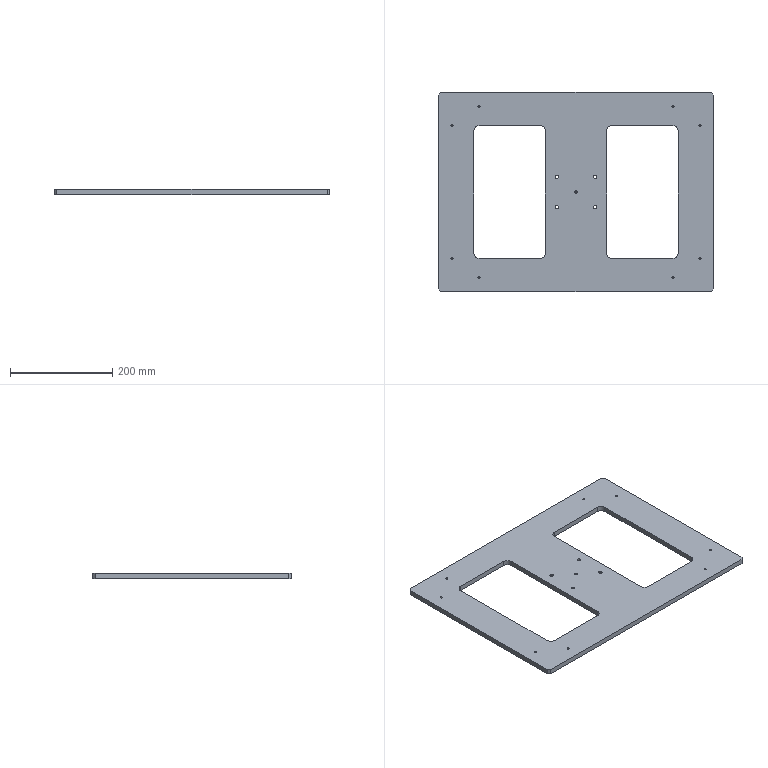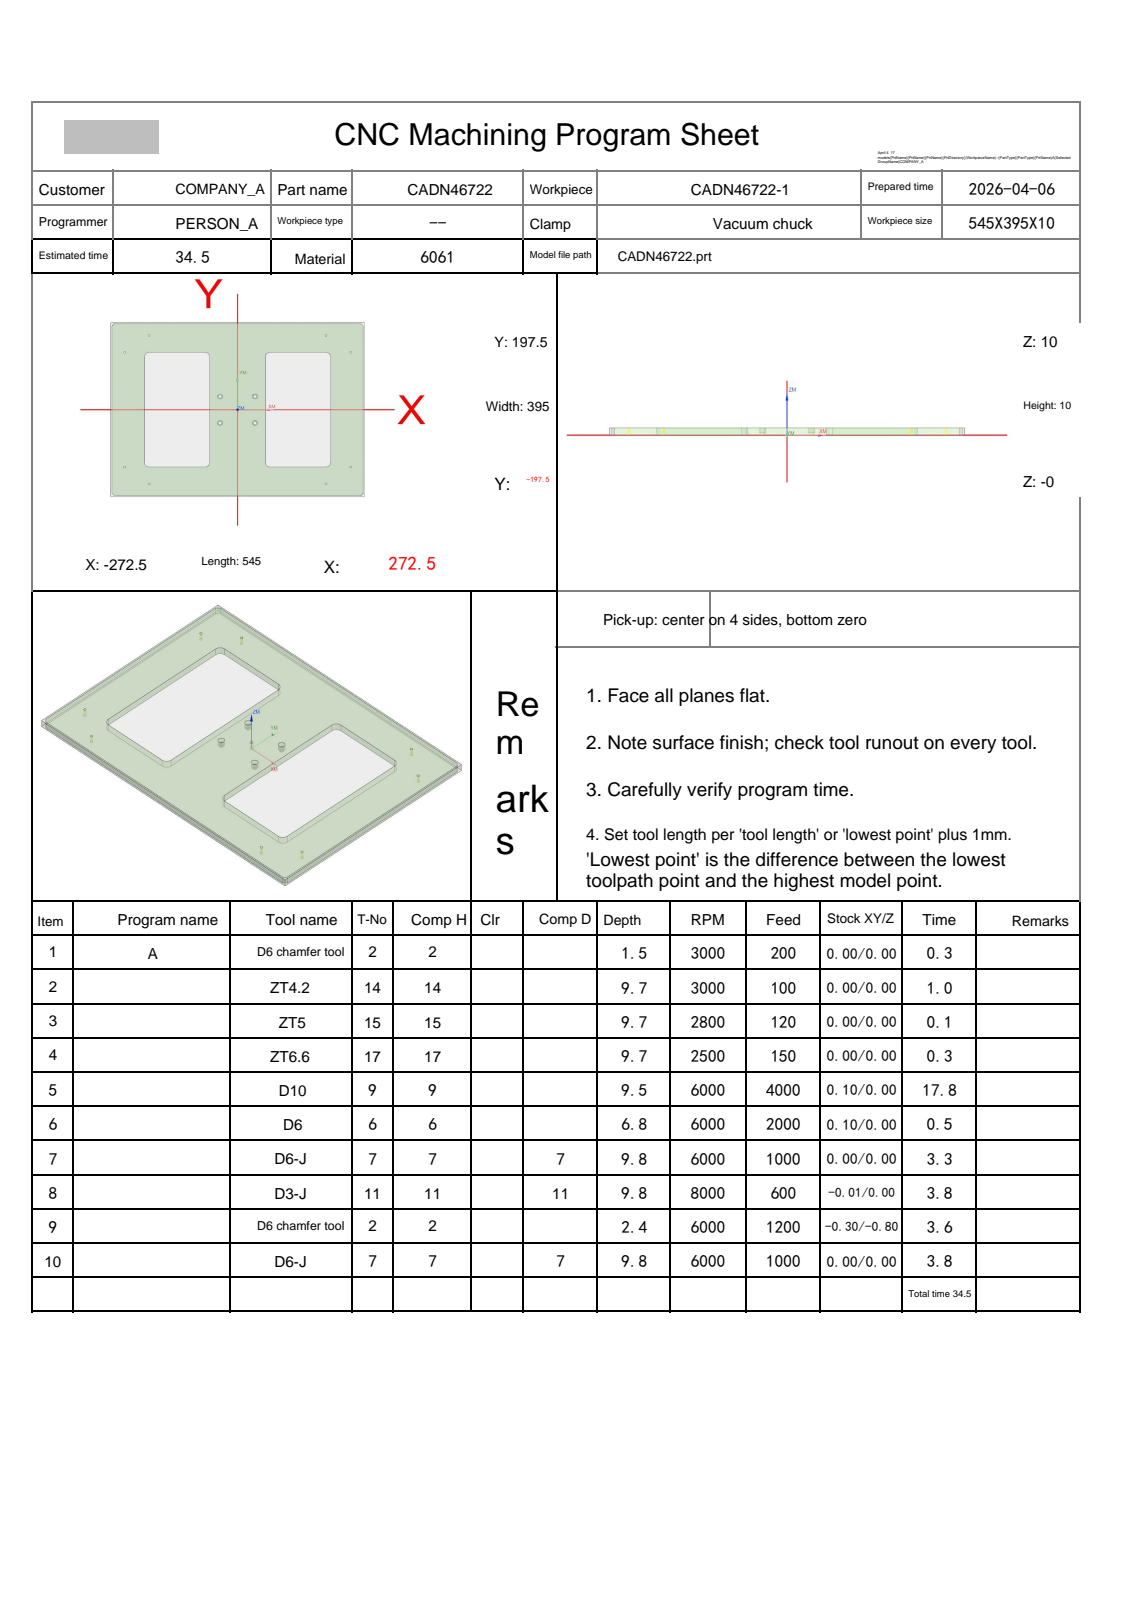NC program | NX | posted by the shop | part box 540 x 390 x 10 mm
Lines 1 to 1058 of 3473:
%
O0001
(Machine time: 36.48 MIN)
(===Total Tool:8===)
(T2=D6 chamfer tool   D=6.   R=0.   D-  H02 Z=7.63  )
(T14=ZT4.2  D=4.2  DR_a=118 D-  H14 Z=0.3   )
(T15=ZT5    D=5.   DR_a=118 D-  H15 Z=0.3   )
(T17=ZT6.6  D=6.6  DR_a=118 D-  H17 Z=0.3   )
(T9=D10     D=10.  R=0.   D-  H09 Z=0.5   )
(T6=D6      D=6.   R=0.   D-  H06 Z=3.2   )
(T7=D6-J    D=6.   R=0.   D7  H07 Z=0.2   )
(T11=D3-J   D=3.   R=0.   D11 H11 Z=0.2   )
G80 G90 G17 G49 G40
G91 G28 Z0
M01
N1 T02 M06
(D6 chamfer tool  D=6. R=0. H=02 ce=0.00 di=0.00)
G00 G90 G54 X190. Y-168. M03 S3000
G43 H02 Z30.
M08
G98 G81 X190. Y-168. Z8.5 R11. F200.
X243. Y-130.
Y130.
X190. Y168.
X37.5 Y30.
Y-30.
X0.0 Y0.0
X-37.5 Y30.
Y-30.
X-190. Y-168.
X-243. Y-130.
Y130.
X-190. Y168.
G80
G00 Z30.
G91 G28 Z0.0
M05
M09
G91 G28 Z0.0
M01
N2 T14 M06
(ZT4.2 D=4.2 DR_a=118 H=14)
G00 G90 G54 X190. Y-168. M03 S3000
G43 H14 Z30.
M08
G98 G83 X190. Y-168. Z.3 R11. F100. Q1.5
X243. Y-130.
Y130.
X190. Y168.
X-190.
X-243. Y130.
Y-130.
X-190. Y-168.
G80
G00 Z30.
G91 G28 Z0.0
M05
M09
G91 G28 Z0.0
M01
N3 T15 M06
(ZT5 D=5. DR_a=118 H=15)
G00 G90 G54 X0.0 Y0.0 M03 S2800
G43 H15 Z30.
M08
G98 G83 X0.0 Y0.0 Z.3 R11. F120. Q1.5
G80
G00 Z30.
G91 G28 Z0.0
M05
M09
G91 G28 Z0.0
M01
N4 T17 M06
(ZT6.6 D=6.6 DR_a=118 H=17)
G00 G90 G54 X-37.5 Y-30. M03 S2500
G43 H17 Z30.
M08
G98 G83 X-37.5 Y-30. Z.3 R11. F150. Q3.
Y30.
X37.5
Y-30.
G80
G00 Z30.
G91 G28 Z0.0
M05
M09
G91 G28 Z0.0
M01
N5 T09 M06
(D10  D=10. R=0. H=09 ce=0.10 di=0.00)
G00 G90 G54 X-194.9 Y0.0 M03 S6000
G43 H09 Z30.
M08
Z10.5
G01 Y-120. Z10.42 F4000.
G03 X-190. Y-124.9 Z10.415 I4.9 J0.0
G01 X-70. Z10.335
G03 X-65.1 Y-120. Z10.33 I0.0 J4.9
G01 Y120. Z10.17
G03 X-70. Y124.9 Z10.165 I-4.9 J0.0
G01 X-190. Z10.085
G03 X-194.9 Y120. Z10.08 I0.0 J-4.9
G01 Y-120. Z9.92
G03 X-190. Y-124.9 Z9.915 I4.9 J0.0
G01 X-70. Z9.835
G03 X-65.1 Y-120. Z9.83 I0.0 J4.9
G01 Y120. Z9.67
G03 X-70. Y124.9 Z9.665 I-4.9 J0.0
G01 X-190. Z9.585
G03 X-194.9 Y120. Z9.58 I0.0 J-4.9
G01 Y-120. Z9.42
G03 X-190. Y-124.9 Z9.415 I4.9 J0.0
G01 X-70. Z9.335
G03 X-65.1 Y-120. Z9.33 I0.0 J4.9
G01 Y120. Z9.17
G03 X-70. Y124.9 Z9.165 I-4.9 J0.0
G01 X-190. Z9.085
G03 X-194.9 Y120. Z9.08 I0.0 J-4.9
G01 Y-120. Z8.92
G03 X-190. Y-124.9 Z8.915 I4.9 J0.0
G01 X-70. Z8.835
G03 X-65.1 Y-120. Z8.83 I0.0 J4.9
G01 Y120. Z8.67
G03 X-70. Y124.9 Z8.665 I-4.9 J0.0
G01 X-190. Z8.585
G03 X-194.9 Y120. Z8.58 I0.0 J-4.9
G01 Y-120. Z8.42
G03 X-190. Y-124.9 Z8.415 I4.9 J0.0
G01 X-70. Z8.335
G03 X-65.1 Y-120. Z8.33 I0.0 J4.9
G01 Y120. Z8.17
G03 X-70. Y124.9 Z8.165 I-4.9 J0.0
G01 X-190. Z8.085
G03 X-194.9 Y120. Z8.08 I0.0 J-4.9
G01 Y-120. Z7.92
G03 X-190. Y-124.9 Z7.915 I4.9 J0.0
G01 X-70. Z7.835
G03 X-65.1 Y-120. Z7.83 I0.0 J4.9
G01 Y120. Z7.67
G03 X-70. Y124.9 Z7.665 I-4.9 J0.0
G01 X-190. Z7.585
G03 X-194.9 Y120. Z7.58 I0.0 J-4.9
G01 Y-120. Z7.42
G03 X-190. Y-124.9 Z7.415 I4.9 J0.0
G01 X-70. Z7.335
G03 X-65.1 Y-120. Z7.33 I0.0 J4.9
G01 Y120. Z7.17
G03 X-70. Y124.9 Z7.165 I-4.9 J0.0
G01 X-190. Z7.085
G03 X-194.9 Y120. Z7.08 I0.0 J-4.9
G01 Y-120. Z6.92
G03 X-190. Y-124.9 Z6.915 I4.9 J0.0
G01 X-70. Z6.835
G03 X-65.1 Y-120. Z6.83 I0.0 J4.9
G01 Y120. Z6.67
G03 X-70. Y124.9 Z6.665 I-4.9 J0.0
G01 X-190. Z6.585
G03 X-194.9 Y120. Z6.58 I0.0 J-4.9
G01 Y-120. Z6.42
G03 X-190. Y-124.9 Z6.415 I4.9 J0.0
G01 X-70. Z6.335
G03 X-65.1 Y-120. Z6.33 I0.0 J4.9
G01 Y120. Z6.17
G03 X-70. Y124.9 Z6.165 I-4.9 J0.0
G01 X-190. Z6.085
G03 X-194.9 Y120. Z6.08 I0.0 J-4.9
G01 Y-120. Z5.92
G03 X-190. Y-124.9 Z5.915 I4.9 J0.0
G01 X-70. Z5.835
G03 X-65.1 Y-120. Z5.83 I0.0 J4.9
G01 Y120. Z5.67
G03 X-70. Y124.9 Z5.665 I-4.9 J0.0
G01 X-190. Z5.585
G03 X-194.9 Y120. Z5.58 I0.0 J-4.9
G01 Y-120. Z5.42
G03 X-190. Y-124.9 Z5.415 I4.9 J0.0
G01 X-70. Z5.335
G03 X-65.1 Y-120. Z5.33 I0.0 J4.9
G01 Y120. Z5.17
G03 X-70. Y124.9 Z5.165 I-4.9 J0.0
G01 X-190. Z5.085
G03 X-194.9 Y120. Z5.08 I0.0 J-4.9
G01 Y-120. Z4.92
G03 X-190. Y-124.9 Z4.915 I4.9 J0.0
G01 X-70. Z4.835
G03 X-65.1 Y-120. Z4.83 I0.0 J4.9
G01 Y120. Z4.67
G03 X-70. Y124.9 Z4.665 I-4.9 J0.0
G01 X-190. Z4.585
G03 X-194.9 Y120. Z4.58 I0.0 J-4.9
G01 Y-120. Z4.42
G03 X-190. Y-124.9 Z4.415 I4.9 J0.0
G01 X-70. Z4.335
G03 X-65.1 Y-120. Z4.33 I0.0 J4.9
G01 Y120. Z4.17
G03 X-70. Y124.9 Z4.165 I-4.9 J0.0
G01 X-190. Z4.085
G03 X-194.9 Y120. Z4.08 I0.0 J-4.9
G01 Y-120. Z3.92
G03 X-190. Y-124.9 Z3.915 I4.9 J0.0
G01 X-70. Z3.835
G03 X-65.1 Y-120. Z3.83 I0.0 J4.9
G01 Y120. Z3.67
G03 X-70. Y124.9 Z3.665 I-4.9 J0.0
G01 X-190. Z3.585
G03 X-194.9 Y120. Z3.58 I0.0 J-4.9
G01 Y-120. Z3.42
G03 X-190. Y-124.9 Z3.415 I4.9 J0.0
G01 X-70. Z3.335
G03 X-65.1 Y-120. Z3.33 I0.0 J4.9
G01 Y120. Z3.17
G03 X-70. Y124.9 Z3.165 I-4.9 J0.0
G01 X-190. Z3.085
G03 X-194.9 Y120. Z3.08 I0.0 J-4.9
G01 Y-120. Z2.92
G03 X-190. Y-124.9 Z2.915 I4.9 J0.0
G01 X-70. Z2.835
G03 X-65.1 Y-120. Z2.83 I0.0 J4.9
G01 Y120. Z2.67
G03 X-70. Y124.9 Z2.665 I-4.9 J0.0
G01 X-190. Z2.585
G03 X-194.9 Y120. Z2.58 I0.0 J-4.9
G01 Y-120. Z2.42
G03 X-190. Y-124.9 Z2.415 I4.9 J0.0
G01 X-70. Z2.335
G03 X-65.1 Y-120. Z2.33 I0.0 J4.9
G01 Y120. Z2.17
G03 X-70. Y124.9 Z2.165 I-4.9 J0.0
G01 X-190. Z2.085
G03 X-194.9 Y120. Z2.08 I0.0 J-4.9
G01 Y-120. Z1.92
G03 X-190. Y-124.9 Z1.915 I4.9 J0.0
G01 X-70. Z1.835
G03 X-65.1 Y-120. Z1.83 I0.0 J4.9
G01 Y120. Z1.67
G03 X-70. Y124.9 Z1.665 I-4.9 J0.0
G01 X-190. Z1.585
G03 X-194.9 Y120. Z1.58 I0.0 J-4.9
G01 Y-120. Z1.42
G03 X-190. Y-124.9 Z1.415 I4.9 J0.0
G01 X-70. Z1.335
G03 X-65.1 Y-120. Z1.33 I0.0 J4.9
G01 Y120. Z1.17
G03 X-70. Y124.9 Z1.165 I-4.9 J0.0
G01 X-190. Z1.085
G03 X-194.9 Y120. Z1.08 I0.0 J-4.9
G01 Y-120. Z.92
G03 X-190. Y-124.9 Z.915 I4.9 J0.0
G01 X-70. Z.835
G03 X-65.1 Y-120. Z.83 I0.0 J4.9
G01 Y120. Z.67
G03 X-70. Y124.9 Z.665 I-4.9 J0.0
G01 X-190. Z.585
G03 X-194.9 Y120. Z.58 I0.0 J-4.9
G01 Y0.0 Z.5
Y-120.
G03 X-190. Y-124.9 I4.9 J0.0
G01 X-70.
G03 X-65.1 Y-120. I0.0 J4.9
G01 Y120.
G03 X-70. Y124.9 I-4.9 J0.0
G01 X-190.
G03 X-194.9 Y120. I0.0 J-4.9
G01 Y0.0
Y-.5
Z1.5
G00 Z30.
X194.9 Y0.0
Z10.5
G01 Y120. Z10.42
G03 X190. Y124.9 Z10.415 I-4.9 J0.0
G01 X70. Z10.335
G03 X65.1 Y120. Z10.33 I0.0 J-4.9
G01 Y-120. Z10.17
G03 X70. Y-124.9 Z10.165 I4.9 J0.0
G01 X190. Z10.085
G03 X194.9 Y-120. Z10.08 I0.0 J4.9
G01 Y120. Z9.92
G03 X190. Y124.9 Z9.915 I-4.9 J0.0
G01 X70. Z9.835
G03 X65.1 Y120. Z9.83 I0.0 J-4.9
G01 Y-120. Z9.67
G03 X70. Y-124.9 Z9.665 I4.9 J0.0
G01 X190. Z9.585
G03 X194.9 Y-120. Z9.58 I0.0 J4.9
G01 Y120. Z9.42
G03 X190. Y124.9 Z9.415 I-4.9 J0.0
G01 X70. Z9.335
G03 X65.1 Y120. Z9.33 I0.0 J-4.9
G01 Y-120. Z9.17
G03 X70. Y-124.9 Z9.165 I4.9 J0.0
G01 X190. Z9.085
G03 X194.9 Y-120. Z9.08 I0.0 J4.9
G01 Y120. Z8.92
G03 X190. Y124.9 Z8.915 I-4.9 J0.0
G01 X70. Z8.835
G03 X65.1 Y120. Z8.83 I0.0 J-4.9
G01 Y-120. Z8.67
G03 X70. Y-124.9 Z8.665 I4.9 J0.0
G01 X190. Z8.585
G03 X194.9 Y-120. Z8.58 I0.0 J4.9
G01 Y120. Z8.42
G03 X190. Y124.9 Z8.415 I-4.9 J0.0
G01 X70. Z8.335
G03 X65.1 Y120. Z8.33 I0.0 J-4.9
G01 Y-120. Z8.17
G03 X70. Y-124.9 Z8.165 I4.9 J0.0
G01 X190. Z8.085
G03 X194.9 Y-120. Z8.08 I0.0 J4.9
G01 Y120. Z7.92
G03 X190. Y124.9 Z7.915 I-4.9 J0.0
G01 X70. Z7.835
G03 X65.1 Y120. Z7.83 I0.0 J-4.9
G01 Y-120. Z7.67
G03 X70. Y-124.9 Z7.665 I4.9 J0.0
G01 X190. Z7.585
G03 X194.9 Y-120. Z7.58 I0.0 J4.9
G01 Y120. Z7.42
G03 X190. Y124.9 Z7.415 I-4.9 J0.0
G01 X70. Z7.335
G03 X65.1 Y120. Z7.33 I0.0 J-4.9
G01 Y-120. Z7.17
G03 X70. Y-124.9 Z7.165 I4.9 J0.0
G01 X190. Z7.085
G03 X194.9 Y-120. Z7.08 I0.0 J4.9
G01 Y120. Z6.92
G03 X190. Y124.9 Z6.915 I-4.9 J0.0
G01 X70. Z6.835
G03 X65.1 Y120. Z6.83 I0.0 J-4.9
G01 Y-120. Z6.67
G03 X70. Y-124.9 Z6.665 I4.9 J0.0
G01 X190. Z6.585
G03 X194.9 Y-120. Z6.58 I0.0 J4.9
G01 Y120. Z6.42
G03 X190. Y124.9 Z6.415 I-4.9 J0.0
G01 X70. Z6.335
G03 X65.1 Y120. Z6.33 I0.0 J-4.9
G01 Y-120. Z6.17
G03 X70. Y-124.9 Z6.165 I4.9 J0.0
G01 X190. Z6.085
G03 X194.9 Y-120. Z6.08 I0.0 J4.9
G01 Y120. Z5.92
G03 X190. Y124.9 Z5.915 I-4.9 J0.0
G01 X70. Z5.835
G03 X65.1 Y120. Z5.83 I0.0 J-4.9
G01 Y-120. Z5.67
G03 X70. Y-124.9 Z5.665 I4.9 J0.0
G01 X190. Z5.585
G03 X194.9 Y-120. Z5.58 I0.0 J4.9
G01 Y120. Z5.42
G03 X190. Y124.9 Z5.415 I-4.9 J0.0
G01 X70. Z5.335
G03 X65.1 Y120. Z5.33 I0.0 J-4.9
G01 Y-120. Z5.17
G03 X70. Y-124.9 Z5.165 I4.9 J0.0
G01 X190. Z5.085
G03 X194.9 Y-120. Z5.08 I0.0 J4.9
G01 Y120. Z4.92
G03 X190. Y124.9 Z4.915 I-4.9 J0.0
G01 X70. Z4.835
G03 X65.1 Y120. Z4.83 I0.0 J-4.9
G01 Y-120. Z4.67
G03 X70. Y-124.9 Z4.665 I4.9 J0.0
G01 X190. Z4.585
G03 X194.9 Y-120. Z4.58 I0.0 J4.9
G01 Y120. Z4.42
G03 X190. Y124.9 Z4.415 I-4.9 J0.0
G01 X70. Z4.335
G03 X65.1 Y120. Z4.33 I0.0 J-4.9
G01 Y-120. Z4.17
G03 X70. Y-124.9 Z4.165 I4.9 J0.0
G01 X190. Z4.085
G03 X194.9 Y-120. Z4.08 I0.0 J4.9
G01 Y120. Z3.92
G03 X190. Y124.9 Z3.915 I-4.9 J0.0
G01 X70. Z3.835
G03 X65.1 Y120. Z3.83 I0.0 J-4.9
G01 Y-120. Z3.67
G03 X70. Y-124.9 Z3.665 I4.9 J0.0
G01 X190. Z3.585
G03 X194.9 Y-120. Z3.58 I0.0 J4.9
G01 Y120. Z3.42
G03 X190. Y124.9 Z3.415 I-4.9 J0.0
G01 X70. Z3.335
G03 X65.1 Y120. Z3.33 I0.0 J-4.9
G01 Y-120. Z3.17
G03 X70. Y-124.9 Z3.165 I4.9 J0.0
G01 X190. Z3.085
G03 X194.9 Y-120. Z3.08 I0.0 J4.9
G01 Y120. Z2.92
G03 X190. Y124.9 Z2.915 I-4.9 J0.0
G01 X70. Z2.835
G03 X65.1 Y120. Z2.83 I0.0 J-4.9
G01 Y-120. Z2.67
G03 X70. Y-124.9 Z2.665 I4.9 J0.0
G01 X190. Z2.585
G03 X194.9 Y-120. Z2.58 I0.0 J4.9
G01 Y120. Z2.42
G03 X190. Y124.9 Z2.415 I-4.9 J0.0
G01 X70. Z2.335
G03 X65.1 Y120. Z2.33 I0.0 J-4.9
G01 Y-120. Z2.17
G03 X70. Y-124.9 Z2.165 I4.9 J0.0
G01 X190. Z2.085
G03 X194.9 Y-120. Z2.08 I0.0 J4.9
G01 Y120. Z1.92
G03 X190. Y124.9 Z1.915 I-4.9 J0.0
G01 X70. Z1.835
G03 X65.1 Y120. Z1.83 I0.0 J-4.9
G01 Y-120. Z1.67
G03 X70. Y-124.9 Z1.665 I4.9 J0.0
G01 X190. Z1.585
G03 X194.9 Y-120. Z1.58 I0.0 J4.9
G01 Y120. Z1.42
G03 X190. Y124.9 Z1.415 I-4.9 J0.0
G01 X70. Z1.335
G03 X65.1 Y120. Z1.33 I0.0 J-4.9
G01 Y-120. Z1.17
G03 X70. Y-124.9 Z1.165 I4.9 J0.0
G01 X190. Z1.085
G03 X194.9 Y-120. Z1.08 I0.0 J4.9
G01 Y120. Z.92
G03 X190. Y124.9 Z.915 I-4.9 J0.0
G01 X70. Z.835
G03 X65.1 Y120. Z.83 I0.0 J-4.9
G01 Y-120. Z.67
G03 X70. Y-124.9 Z.665 I4.9 J0.0
G01 X190. Z.585
G03 X194.9 Y-120. Z.58 I0.0 J4.9
G01 Y0.0 Z.5
Y120.
G03 X190. Y124.9 I-4.9 J0.0
G01 X70.
G03 X65.1 Y120. I0.0 J-4.9
G01 Y-120.
G03 X70. Y-124.9 I4.9 J0.0
G01 X190.
G03 X194.9 Y-120. I0.0 J4.9
G01 Y0.0
Y.5
Z1.5
G00 Z30.
G00 G90 X0.0 Y-200.1 M03 S6000
Z30.
Z10.5
G01 X-265. Z10.43 F4000.
G02 X-268.606 Y-198.606 Z10.428 I0.0 J5.1
G01 X-273.606 Y-193.606 Z10.427
G02 X-275.1 Y-190. Z10.426 I3.606 J3.606
G01 Y190. Z10.324
G02 X-273.606 Y193.606 Z10.323 I5.1 J0.0
G01 X-268.606 Y198.606 Z10.322
G02 X-265. Y200.1 Z10.32 I3.606 J-3.606
G01 X265. Z10.18
G02 X268.606 Y198.606 Z10.178 I0.0 J-5.1
G01 X273.606 Y193.606 Z10.177
G02 X275.1 Y190. Z10.176 I-3.606 J-3.606
G01 Y-190. Z10.074
G02 X273.606 Y-193.606 Z10.073 I-5.1 J0.0
G01 X268.606 Y-198.606 Z10.072
G02 X265. Y-200.1 Z10.07 I-3.606 J3.606
G01 X-265. Z9.93
G02 X-268.606 Y-198.606 Z9.928 I0.0 J5.1
G01 X-273.606 Y-193.606 Z9.927
G02 X-275.1 Y-190. Z9.926 I3.606 J3.606
G01 Y190. Z9.824
G02 X-273.606 Y193.606 Z9.823 I5.1 J0.0
G01 X-268.606 Y198.606 Z9.822
G02 X-265. Y200.1 Z9.82 I3.606 J-3.606
G01 X265. Z9.68
G02 X268.606 Y198.606 Z9.678 I0.0 J-5.1
G01 X273.606 Y193.606 Z9.677
G02 X275.1 Y190. Z9.676 I-3.606 J-3.606
G01 Y-190. Z9.574
G02 X273.606 Y-193.606 Z9.573 I-5.1 J0.0
G01 X268.606 Y-198.606 Z9.572
G02 X265. Y-200.1 Z9.57 I-3.606 J3.606
G01 X-265. Z9.43
G02 X-268.606 Y-198.606 Z9.428 I0.0 J5.1
G01 X-273.606 Y-193.606 Z9.427
G02 X-275.1 Y-190. Z9.426 I3.606 J3.606
G01 Y190. Z9.324
G02 X-273.606 Y193.606 Z9.323 I5.1 J0.0
G01 X-268.606 Y198.606 Z9.322
G02 X-265. Y200.1 Z9.32 I3.606 J-3.606
G01 X265. Z9.18
G02 X268.606 Y198.606 Z9.178 I0.0 J-5.1
G01 X273.606 Y193.606 Z9.177
G02 X275.1 Y190. Z9.176 I-3.606 J-3.606
G01 Y-190. Z9.074
G02 X273.606 Y-193.606 Z9.073 I-5.1 J0.0
G01 X268.606 Y-198.606 Z9.072
G02 X265. Y-200.1 Z9.07 I-3.606 J3.606
G01 X-265. Z8.93
G02 X-268.606 Y-198.606 Z8.928 I0.0 J5.1
G01 X-273.606 Y-193.606 Z8.927
G02 X-275.1 Y-190. Z8.926 I3.606 J3.606
G01 Y190. Z8.824
G02 X-273.606 Y193.606 Z8.823 I5.1 J0.0
G01 X-268.606 Y198.606 Z8.822
G02 X-265. Y200.1 Z8.82 I3.606 J-3.606
G01 X265. Z8.68
G02 X268.606 Y198.606 Z8.678 I0.0 J-5.1
G01 X273.606 Y193.606 Z8.677
G02 X275.1 Y190. Z8.676 I-3.606 J-3.606
G01 Y-190. Z8.574
G02 X273.606 Y-193.606 Z8.573 I-5.1 J0.0
G01 X268.606 Y-198.606 Z8.572
G02 X265. Y-200.1 Z8.57 I-3.606 J3.606
G01 X-265. Z8.43
G02 X-268.606 Y-198.606 Z8.428 I0.0 J5.1
G01 X-273.606 Y-193.606 Z8.427
G02 X-275.1 Y-190. Z8.426 I3.606 J3.606
G01 Y190. Z8.324
G02 X-273.606 Y193.606 Z8.323 I5.1 J0.0
G01 X-268.606 Y198.606 Z8.322
G02 X-265. Y200.1 Z8.32 I3.606 J-3.606
G01 X265. Z8.18
G02 X268.606 Y198.606 Z8.178 I0.0 J-5.1
G01 X273.606 Y193.606 Z8.177
G02 X275.1 Y190. Z8.176 I-3.606 J-3.606
G01 Y-190. Z8.074
G02 X273.606 Y-193.606 Z8.073 I-5.1 J0.0
G01 X268.606 Y-198.606 Z8.072
G02 X265. Y-200.1 Z8.07 I-3.606 J3.606
G01 X-265. Z7.93
G02 X-268.606 Y-198.606 Z7.928 I0.0 J5.1
G01 X-273.606 Y-193.606 Z7.927
G02 X-275.1 Y-190. Z7.926 I3.606 J3.606
G01 Y190. Z7.824
G02 X-273.606 Y193.606 Z7.823 I5.1 J0.0
G01 X-268.606 Y198.606 Z7.822
G02 X-265. Y200.1 Z7.82 I3.606 J-3.606
G01 X265. Z7.68
G02 X268.606 Y198.606 Z7.678 I0.0 J-5.1
G01 X273.606 Y193.606 Z7.677
G02 X275.1 Y190. Z7.676 I-3.606 J-3.606
G01 Y-190. Z7.574
G02 X273.606 Y-193.606 Z7.573 I-5.1 J0.0
G01 X268.606 Y-198.606 Z7.572
G02 X265. Y-200.1 Z7.57 I-3.606 J3.606
G01 X-265. Z7.43
G02 X-268.606 Y-198.606 Z7.428 I0.0 J5.1
G01 X-273.606 Y-193.606 Z7.427
G02 X-275.1 Y-190. Z7.426 I3.606 J3.606
G01 Y190. Z7.324
G02 X-273.606 Y193.606 Z7.323 I5.1 J0.0
G01 X-268.606 Y198.606 Z7.322
G02 X-265. Y200.1 Z7.32 I3.606 J-3.606
G01 X265. Z7.18
G02 X268.606 Y198.606 Z7.178 I0.0 J-5.1
G01 X273.606 Y193.606 Z7.177
G02 X275.1 Y190. Z7.176 I-3.606 J-3.606
G01 Y-190. Z7.074
G02 X273.606 Y-193.606 Z7.073 I-5.1 J0.0
G01 X268.606 Y-198.606 Z7.072
G02 X265. Y-200.1 Z7.07 I-3.606 J3.606
G01 X-265. Z6.93
G02 X-268.606 Y-198.606 Z6.928 I0.0 J5.1
G01 X-273.606 Y-193.606 Z6.927
G02 X-275.1 Y-190. Z6.926 I3.606 J3.606
G01 Y190. Z6.824
G02 X-273.606 Y193.606 Z6.823 I5.1 J0.0
G01 X-268.606 Y198.606 Z6.822
G02 X-265. Y200.1 Z6.82 I3.606 J-3.606
G01 X265. Z6.68
G02 X268.606 Y198.606 Z6.678 I0.0 J-5.1
G01 X273.606 Y193.606 Z6.677
G02 X275.1 Y190. Z6.676 I-3.606 J-3.606
G01 Y-190. Z6.574
G02 X273.606 Y-193.606 Z6.573 I-5.1 J0.0
G01 X268.606 Y-198.606 Z6.572
G02 X265. Y-200.1 Z6.57 I-3.606 J3.606
G01 X-265. Z6.43
G02 X-268.606 Y-198.606 Z6.428 I0.0 J5.1
G01 X-273.606 Y-193.606 Z6.427
G02 X-275.1 Y-190. Z6.426 I3.606 J3.606
G01 Y190. Z6.324
G02 X-273.606 Y193.606 Z6.323 I5.1 J0.0
G01 X-268.606 Y198.606 Z6.322
G02 X-265. Y200.1 Z6.32 I3.606 J-3.606
G01 X265. Z6.18
G02 X268.606 Y198.606 Z6.178 I0.0 J-5.1
G01 X273.606 Y193.606 Z6.177
G02 X275.1 Y190. Z6.176 I-3.606 J-3.606
G01 Y-190. Z6.074
G02 X273.606 Y-193.606 Z6.073 I-5.1 J0.0
G01 X268.606 Y-198.606 Z6.072
G02 X265. Y-200.1 Z6.07 I-3.606 J3.606
G01 X-265. Z5.93
G02 X-268.606 Y-198.606 Z5.928 I0.0 J5.1
G01 X-273.606 Y-193.606 Z5.927
G02 X-275.1 Y-190. Z5.926 I3.606 J3.606
G01 Y190. Z5.824
G02 X-273.606 Y193.606 Z5.823 I5.1 J0.0
G01 X-268.606 Y198.606 Z5.822
G02 X-265. Y200.1 Z5.82 I3.606 J-3.606
G01 X265. Z5.68
G02 X268.606 Y198.606 Z5.678 I0.0 J-5.1
G01 X273.606 Y193.606 Z5.677
G02 X275.1 Y190. Z5.676 I-3.606 J-3.606
G01 Y-190. Z5.574
G02 X273.606 Y-193.606 Z5.573 I-5.1 J0.0
G01 X268.606 Y-198.606 Z5.572
G02 X265. Y-200.1 Z5.57 I-3.606 J3.606
G01 X-265. Z5.43
G02 X-268.606 Y-198.606 Z5.428 I0.0 J5.1
G01 X-273.606 Y-193.606 Z5.427
G02 X-275.1 Y-190. Z5.426 I3.606 J3.606
G01 Y190. Z5.324
G02 X-273.606 Y193.606 Z5.323 I5.1 J0.0
G01 X-268.606 Y198.606 Z5.322
G02 X-265. Y200.1 Z5.32 I3.606 J-3.606
G01 X265. Z5.18
G02 X268.606 Y198.606 Z5.178 I0.0 J-5.1
G01 X273.606 Y193.606 Z5.177
G02 X275.1 Y190. Z5.176 I-3.606 J-3.606
G01 Y-190. Z5.074
G02 X273.606 Y-193.606 Z5.073 I-5.1 J0.0
G01 X268.606 Y-198.606 Z5.072
G02 X265. Y-200.1 Z5.07 I-3.606 J3.606
G01 X-265. Z4.93
G02 X-268.606 Y-198.606 Z4.928 I0.0 J5.1
G01 X-273.606 Y-193.606 Z4.927
G02 X-275.1 Y-190. Z4.926 I3.606 J3.606
G01 Y190. Z4.824
G02 X-273.606 Y193.606 Z4.823 I5.1 J0.0
G01 X-268.606 Y198.606 Z4.822
G02 X-265. Y200.1 Z4.82 I3.606 J-3.606
G01 X265. Z4.68
G02 X268.606 Y198.606 Z4.678 I0.0 J-5.1
G01 X273.606 Y193.606 Z4.677
G02 X275.1 Y190. Z4.676 I-3.606 J-3.606
G01 Y-190. Z4.574
G02 X273.606 Y-193.606 Z4.573 I-5.1 J0.0
G01 X268.606 Y-198.606 Z4.572
G02 X265. Y-200.1 Z4.57 I-3.606 J3.606
G01 X-265. Z4.43
G02 X-268.606 Y-198.606 Z4.428 I0.0 J5.1
G01 X-273.606 Y-193.606 Z4.427
G02 X-275.1 Y-190. Z4.426 I3.606 J3.606
G01 Y190. Z4.324
G02 X-273.606 Y193.606 Z4.323 I5.1 J0.0
G01 X-268.606 Y198.606 Z4.322
G02 X-265. Y200.1 Z4.32 I3.606 J-3.606
G01 X265. Z4.18
G02 X268.606 Y198.606 Z4.178 I0.0 J-5.1
G01 X273.606 Y193.606 Z4.177
G02 X275.1 Y190. Z4.176 I-3.606 J-3.606
G01 Y-190. Z4.074
G02 X273.606 Y-193.606 Z4.073 I-5.1 J0.0
G01 X268.606 Y-198.606 Z4.072
G02 X265. Y-200.1 Z4.07 I-3.606 J3.606
G01 X-265. Z3.93
G02 X-268.606 Y-198.606 Z3.928 I0.0 J5.1
G01 X-273.606 Y-193.606 Z3.927
G02 X-275.1 Y-190. Z3.926 I3.606 J3.606
G01 Y190. Z3.824
G02 X-273.606 Y193.606 Z3.823 I5.1 J0.0
G01 X-268.606 Y198.606 Z3.822
G02 X-265. Y200.1 Z3.82 I3.606 J-3.606
G01 X265. Z3.68
G02 X268.606 Y198.606 Z3.678 I0.0 J-5.1
G01 X273.606 Y193.606 Z3.677
G02 X275.1 Y190. Z3.676 I-3.606 J-3.606
G01 Y-190. Z3.574
G02 X273.606 Y-193.606 Z3.573 I-5.1 J0.0
G01 X268.606 Y-198.606 Z3.572
G02 X265. Y-200.1 Z3.57 I-3.606 J3.606
G01 X-265. Z3.43
G02 X-268.606 Y-198.606 Z3.428 I0.0 J5.1
G01 X-273.606 Y-193.606 Z3.427
G02 X-275.1 Y-190. Z3.426 I3.606 J3.606
G01 Y190. Z3.324
G02 X-273.606 Y193.606 Z3.323 I5.1 J0.0
G01 X-268.606 Y198.606 Z3.322
G02 X-265. Y200.1 Z3.32 I3.606 J-3.606
G01 X265. Z3.18
G02 X268.606 Y198.606 Z3.178 I0.0 J-5.1
G01 X273.606 Y193.606 Z3.177
G02 X275.1 Y190. Z3.176 I-3.606 J-3.606
G01 Y-190. Z3.074
G02 X273.606 Y-193.606 Z3.073 I-5.1 J0.0
G01 X268.606 Y-198.606 Z3.072
G02 X265. Y-200.1 Z3.07 I-3.606 J3.606
G01 X-265. Z2.93
G02 X-268.606 Y-198.606 Z2.928 I0.0 J5.1
G01 X-273.606 Y-193.606 Z2.927
G02 X-275.1 Y-190. Z2.926 I3.606 J3.606
G01 Y190. Z2.824
G02 X-273.606 Y193.606 Z2.823 I5.1 J0.0
G01 X-268.606 Y198.606 Z2.822
G02 X-265. Y200.1 Z2.82 I3.606 J-3.606
G01 X265. Z2.68
G02 X268.606 Y198.606 Z2.678 I0.0 J-5.1
G01 X273.606 Y193.606 Z2.677
G02 X275.1 Y190. Z2.676 I-3.606 J-3.606
G01 Y-190. Z2.574
G02 X273.606 Y-193.606 Z2.573 I-5.1 J0.0
G01 X268.606 Y-198.606 Z2.572
G02 X265. Y-200.1 Z2.57 I-3.606 J3.606
G01 X-265. Z2.43
G02 X-268.606 Y-198.606 Z2.428 I0.0 J5.1
G01 X-273.606 Y-193.606 Z2.427
G02 X-275.1 Y-190. Z2.426 I3.606 J3.606
G01 Y190. Z2.324
G02 X-273.606 Y193.606 Z2.323 I5.1 J0.0
G01 X-268.606 Y198.606 Z2.322
G02 X-265. Y200.1 Z2.32 I3.606 J-3.606
G01 X265. Z2.18
G02 X268.606 Y198.606 Z2.178 I0.0 J-5.1
G01 X273.606 Y193.606 Z2.177
G02 X275.1 Y190. Z2.176 I-3.606 J-3.606
G01 Y-190. Z2.074
G02 X273.606 Y-193.606 Z2.073 I-5.1 J0.0
G01 X268.606 Y-198.606 Z2.072
G02 X265. Y-200.1 Z2.07 I-3.606 J3.606
G01 X-265. Z1.93
G02 X-268.606 Y-198.606 Z1.928 I0.0 J5.1
G01 X-273.606 Y-193.606 Z1.927
G02 X-275.1 Y-190. Z1.926 I3.606 J3.606
G01 Y190. Z1.824
G02 X-273.606 Y193.606 Z1.823 I5.1 J0.0
G01 X-268.606 Y198.606 Z1.822
G02 X-265. Y200.1 Z1.82 I3.606 J-3.606
G01 X265. Z1.68
G02 X268.606 Y198.606 Z1.678 I0.0 J-5.1
G01 X273.606 Y193.606 Z1.677
G02 X275.1 Y190. Z1.676 I-3.606 J-3.606
G01 Y-190. Z1.574
G02 X273.606 Y-193.606 Z1.573 I-5.1 J0.0
G01 X268.606 Y-198.606 Z1.572
G02 X265. Y-200.1 Z1.57 I-3.606 J3.606
G01 X-265. Z1.43
G02 X-268.606 Y-198.606 Z1.428 I0.0 J5.1
G01 X-273.606 Y-193.606 Z1.427
G02 X-275.1 Y-190. Z1.426 I3.606 J3.606
G01 Y190. Z1.324
G02 X-273.606 Y193.606 Z1.323 I5.1 J0.0
G01 X-268.606 Y198.606 Z1.322
G02 X-265. Y200.1 Z1.32 I3.606 J-3.606
G01 X265. Z1.18
G02 X268.606 Y198.606 Z1.178 I0.0 J-5.1
G01 X273.606 Y193.606 Z1.177
G02 X275.1 Y190. Z1.176 I-3.606 J-3.606
G01 Y-190. Z1.074
G02 X273.606 Y-193.606 Z1.073 I-5.1 J0.0
G01 X268.606 Y-198.606 Z1.072
G02 X265. Y-200.1 Z1.07 I-3.606 J3.606
G01 X-265. Z.93
G02 X-268.606 Y-198.606 Z.928 I0.0 J5.1
G01 X-273.606 Y-193.606 Z.927
G02 X-275.1 Y-190. Z.926 I3.606 J3.606
G01 Y190. Z.824
G02 X-273.606 Y193.606 Z.823 I5.1 J0.0
G01 X-268.606 Y198.606 Z.822
G02 X-265. Y200.1 Z.82 I3.606 J-3.606
G01 X265. Z.68
G02 X268.606 Y198.606 Z.678 I0.0 J-5.1
G01 X273.606 Y193.606 Z.677
G02 X275.1 Y190. Z.676 I-3.606 J-3.606
G01 Y-190. Z.574
G02 X273.606 Y-193.606 Z.573 I-5.1 J0.0
G01 X268.606 Y-198.606 Z.572
G02 X265. Y-200.1 Z.57 I-3.606 J3.606
G01 X0.0 Z.5
X-265.
G02 X-268.606 Y-198.606 I0.0 J5.1
G01 X-273.606 Y-193.606
G02 X-275.1 Y-190. I3.606 J3.606
G01 Y190.
G02 X-273.606 Y193.606 I5.1 J0.0
G01 X-268.606 Y198.606
G02 X-265. Y200.1 I3.606 J-3.606
G01 X265.
G02 X268.606 Y198.606 I0.0 J-5.1
G01 X273.606 Y193.606
G02 X275.1 Y190. I-3.606 J-3.606
G01 Y-190.
G02 X273.606 Y-193.606 I-5.1 J0.0
G01 X268.606 Y-198.606
G02 X265. Y-200.1 I-3.606 J3.606
G01 X0.0
X-.5
Z1.5
G00 Z30.
G91 G28 Z0.0
M05
M09
G91 G28 Z0.0
M01
N6 T06 M06
(D6  D=6. R=0. H=06 ce=0.10 di=0.00)
G00 G90 G54 X-37.5 Y-30. M03 S6000
G43 H06 Z30.
M08
Z10.3
G03 X-36.3 Y-31.2 I1.2 J0.0 F2000.
X-35.1 Y-30. I0.0 J1.2
X-35.1 Y-30. Z9.8 I-2.4 J0.0
X-35.1 Y-30. Z9.3 I-2.4 J0.0
X-35.1 Y-30. Z8.8 I-2.4 J0.0
X-35.1 Y-30. Z8.3 I-2.4 J0.0
X-35.1 Y-30. Z7.8 I-2.4 J0.0
X-35.1 Y-30. Z7.3 I-2.4 J0.0
X-35.1 Y-30. Z6.8 I-2.4 J0.0
X-35.1 Y-30. Z6.3 I-2.4 J0.0
X-35.1 Y-30. Z5.8 I-2.4 J0.0
X-35.1 Y-30. Z5.3 I-2.4 J0.0
X-35.1 Y-30. Z4.8 I-2.4 J0.0
X-35.1 Y-30. Z4.3 I-2.4 J0.0
X-35.1 Y-30. Z3.8 I-2.4 J0.0
X-35.1 Y-30. Z3.3 I-2.4 J0.0
X-36.758 Y-27.717 Z3.2 I-2.4 J0.0
X-37.5 Y-27.6 I-.742 J-2.283
X-39.9 Y-30. I0.0 J-2.4
X-37.5 Y-32.4 I2.4 J0.0
X-35.1 Y-30. I0.0 J2.4
X-36.758 Y-27.717 I-2.4 J0.0
X-37.129 Y-27.659 I-.371 J-1.141
X-38.329 Y-28.859 I0.0 J-1.2
X-37.5 Y-30. I1.2 J0.0
G00 Z30.
Y30.
Z10.3
G03 X-36.3 Y28.8 I1.2 J0.0
X-35.1 Y30. I0.0 J1.2
X-35.1 Y30. Z9.8 I-2.4 J0.0
X-35.1 Y30. Z9.3 I-2.4 J0.0
X-35.1 Y30. Z8.8 I-2.4 J0.0
X-35.1 Y30. Z8.3 I-2.4 J0.0
X-35.1 Y30. Z7.8 I-2.4 J0.0
X-35.1 Y30. Z7.3 I-2.4 J0.0
X-35.1 Y30. Z6.8 I-2.4 J0.0
X-35.1 Y30. Z6.3 I-2.4 J0.0
X-35.1 Y30. Z5.8 I-2.4 J0.0
X-35.1 Y30. Z5.3 I-2.4 J0.0
X-35.1 Y30. Z4.8 I-2.4 J0.0
X-35.1 Y30. Z4.3 I-2.4 J0.0
X-35.1 Y30. Z3.8 I-2.4 J0.0
X-35.1 Y30. Z3.3 I-2.4 J0.0
X-36.758 Y32.283 Z3.2 I-2.4 J0.0
X-37.5 Y32.4 I-.742 J-2.283
X-39.9 Y30. I0.0 J-2.4
X-37.5 Y27.6 I2.4 J0.0
X-35.1 Y30. I0.0 J2.4
X-36.758 Y32.283 I-2.4 J0.0
X-37.129 Y32.341 I-.371 J-1.141
X-38.329 Y31.141 I0.0 J-1.2
X-37.5 Y30. I1.2 J0.0
G00 Z30.
X37.5
Z10.3
G03 X38.7 Y28.8 I1.2 J0.0
X39.9 Y30. I0.0 J1.2
X39.9 Y30. Z9.8 I-2.4 J0.0
X39.9 Y30. Z9.3 I-2.4 J0.0
X39.9 Y30. Z8.8 I-2.4 J0.0
X39.9 Y30. Z8.3 I-2.4 J0.0
X39.9 Y30. Z7.8 I-2.4 J0.0
X39.9 Y30. Z7.3 I-2.4 J0.0
X39.9 Y30. Z6.8 I-2.4 J0.0
X39.9 Y30. Z6.3 I-2.4 J0.0
X39.9 Y30. Z5.8 I-2.4 J0.0
X39.9 Y30. Z5.3 I-2.4 J0.0
X39.9 Y30. Z4.8 I-2.4 J0.0
X39.9 Y30. Z4.3 I-2.4 J0.0
X39.9 Y30. Z3.8 I-2.4 J0.0
X39.9 Y30. Z3.3 I-2.4 J0.0
X38.242 Y32.283 Z3.2 I-2.4 J0.0
X37.5 Y32.4 I-.742 J-2.283
X35.1 Y30. I0.0 J-2.4
X37.5 Y27.6 I2.4 J0.0
X39.9 Y30. I0.0 J2.4
X38.242 Y32.283 I-2.4 J0.0
X37.871 Y32.341 I-.371 J-1.141
X36.671 Y31.141 I0.0 J-1.2
X37.5 Y30. I1.2 J0.0
G00 Z30.
Y-30.
Z10.3
G03 X38.7 Y-31.2 I1.2 J0.0
X39.9 Y-30. I0.0 J1.2
X39.9 Y-30. Z9.8 I-2.4 J0.0
X39.9 Y-30. Z9.3 I-2.4 J0.0
X39.9 Y-30. Z8.8 I-2.4 J0.0
X39.9 Y-30. Z8.3 I-2.4 J0.0
X39.9 Y-30. Z7.8 I-2.4 J0.0
X39.9 Y-30. Z7.3 I-2.4 J0.0
X39.9 Y-30. Z6.8 I-2.4 J0.0
X39.9 Y-30. Z6.3 I-2.4 J0.0
X39.9 Y-30. Z5.8 I-2.4 J0.0
X39.9 Y-30. Z5.3 I-2.4 J0.0
X39.9 Y-30. Z4.8 I-2.4 J0.0
X39.9 Y-30. Z4.3 I-2.4 J0.0
X39.9 Y-30. Z3.8 I-2.4 J0.0
X39.9 Y-30. Z3.3 I-2.4 J0.0
X38.242 Y-27.717 Z3.2 I-2.4 J0.0
X37.5 Y-27.6 I-.742 J-2.283
X35.1 Y-30. I0.0 J-2.4
X37.5 Y-32.4 I2.4 J0.0
X39.9 Y-30. I0.0 J2.4
X38.242 Y-27.717 I-2.4 J0.0
X37.871 Y-27.659 I-.371 J-1.141
X36.671 Y-28.859 I0.0 J-1.2
X37.5 Y-30. I1.2 J0.0
G00 Z30.
G91 G28 Z0.0
M05
M09
G91 G28 Z0.0
M01
N7 T07 M06
(D6-J  D=6. R=0. H=07 ce=0.00 di=0.00)
G00 G90 G54 X195.716 Y-121. M03 S6000
G43 H07 Z30.
M08
Z1.
G01 Z.5 F1000.
G41 D07
X196.
G03 X197. Y-120. I0.0 J1.
G01 Y120.
G03 X190. Y127. I-7. J0.0
G01 X70.
G03 X63. Y120. I0.0 J-7.
G01 Y-120.
G03 X70. Y-127. I7. J0.0
G01 X190.
G03 X197. Y-120. I0.0 J7.
G01 Y-119.5
G03 X196. Y-118.5 I-1. J0.0
G01 G40 X195.8
Z1.
G00 Z30.
X-195.716 Y121.
Z1.
G01 Z.5
G41 D07
X-196.
G03 X-197. Y120. I0.0 J-1.
G01 Y-120.
G03 X-190. Y-127. I7. J0.0
G01 X-70.
G03 X-63. Y-120. I0.0 J7.
G01 Y120.
G03 X-70. Y127. I-7. J0.0
G01 X-190.
G03 X-197. Y120. I0.0 J-7.
G01 Y119.5
G03 X-196. Y118.5 I1. J0.0
G01 G40 X-195.8
Z1.
G00 Z30.
G00 G90 X195.816 Y-121. M03 S6000
Z30.
Z.7
G01 Z.2 F1000.
G41 D07
X196.
G03 X197. Y-120. I0.0 J1.
G01 Y120.
G03 X190. Y127. I-7. J0.0
G01 X70.
G03 X63. Y120. I0.0 J-7.
G01 Y-120.
G03 X70. Y-127. I7. J0.0
G01 X190.
G03 X197. Y-120. I0.0 J7.
G01 Y-119.5
G03 X196. Y-118.5 I-1. J0.0
G01 G40 X195.9
Z.7
G00 Z30.
X-195.816 Y121.
Z.7
G01 Z.2
G41 D07
X-196.
G03 X-197. Y120. I0.0 J-1.
G01 Y-120.
G03 X-190. Y-127. I7. J0.0
G01 X-70.
G03 X-63. Y-120. I0.0 J7.
G01 Y120.
G03 X-70. Y127. I-7. J0.0
G01 X-190.
G03 X-197. Y120. I0.0 J-7.
G01 Y119.5
G03 X-196. Y118.5 I1. J0.0
G01 G40 X-195.9
Z.7
G00 Z30.
G00 G90 X-37.5 Y-30. M03 S6000
Z30.
Z3.2
G01 X-35.432 Y-30.362 F800.
X-35.368 Y-30.368
G03 X-35. Y-30. I0.0 J.368
X-37.5 Y-27.5 I-2.5 J0.0
X-40. Y-30. I0.0 J-2.5
X-37.5 Y-32.5 I2.5 J0.0
X-35. Y-30. I0.0 J2.5
X-35.05 Y-29.503 I-2.5 J0.0
X-35.41 Y-29.208 I-.361 J-.073
G01 X-35.545 Y-29.234
X-37.5 Y-30.
G00 Z30.
Y30.
Z3.2
G01 X-35.432 Y29.638
X-35.368 Y29.632
G03 X-35. Y30. I0.0 J.368
X-37.5 Y32.5 I-2.5 J0.0
X-40. Y30. I0.0 J-2.5
X-37.5 Y27.5 I2.5 J0.0
X-35. Y30. I0.0 J2.5
X-35.05 Y30.497 I-2.5 J0.0
X-35.41 Y30.792 I-.361 J-.073
G01 X-35.545 Y30.766
X-37.5 Y30.
G00 Z30.
X37.5
Z3.2
G01 X39.568 Y29.638
X39.632 Y29.632
G03 X40. Y30. I0.0 J.368
X37.5 Y32.5 I-2.5 J0.0
X35. Y30. I0.0 J-2.5
X37.5 Y27.5 I2.5 J0.0
X40. Y30. I0.0 J2.5
X39.95 Y30.497 I-2.5 J0.0
X39.59 Y30.792 I-.361 J-.073
G01 X39.455 Y30.766
X37.5 Y30.
G00 Z30.
Y-30.
Z3.2
G01 X39.568 Y-30.362
X39.632 Y-30.368
G03 X40. Y-30. I0.0 J.368
X37.5 Y-27.5 I-2.5 J0.0
X35. Y-30. I0.0 J-2.5
X37.5 Y-32.5 I2.5 J0.0
X40. Y-30. I0.0 J2.5
X39.95 Y-29.503 I-2.5 J0.0
X39.59 Y-29.208 I-.361 J-.073
G01 X39.455 Y-29.234
X37.5 Y-30.
G00 Z30.
G91 G28 Z0.0
M05
M09
G91 G28 Z0.0
M01